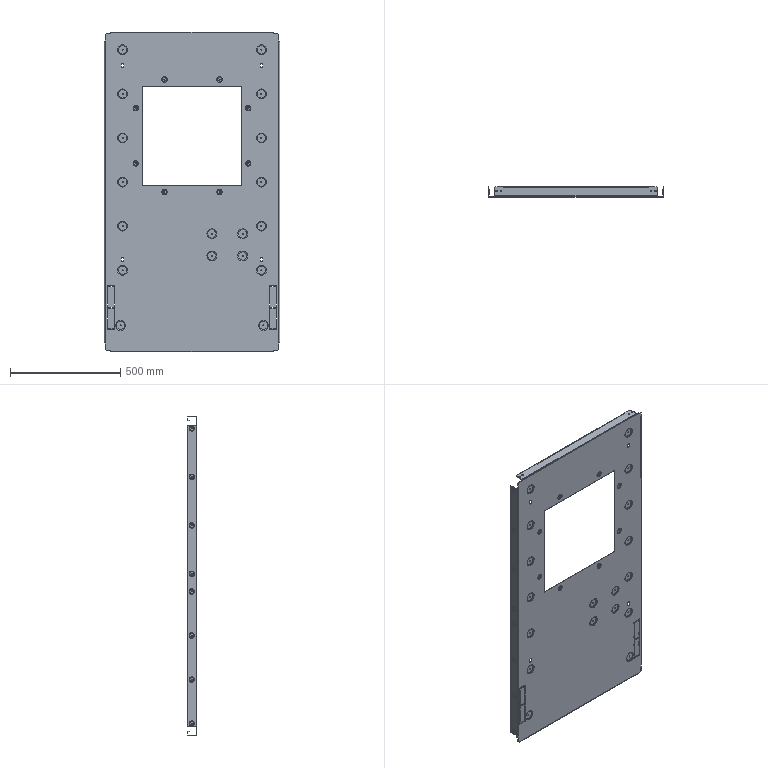Part | STEP file | 1 solid | 902 faces | box 796 x 45 x 1450 mm | volume 2326374 mm3 | torus 336 | cylinder 296 | plane 270 | commonest cylinder face diameters 4.7 x84 20 x48 24 x48 40 x36 44 x36 7 x24